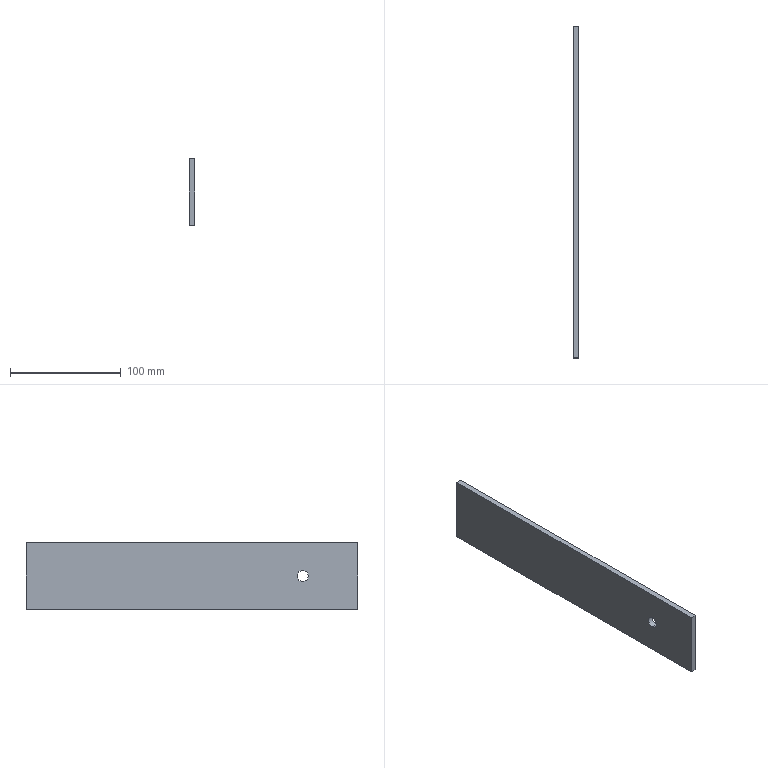Part | SolidWorks | features Extrusion 1, ICE 1 | 1 solid | 8 faces | box 5 x 300 x 60 mm | volume 89607 mm3 | plane 6 | cylinder 2 | commonest cylinder face diameters 10 x2
STEP:
#1=CARTESIAN_POINT('',(-2.5,-100.,35.));
#2=VERTEX_POINT('',#1);
#3=CARTESIAN_POINT('',(-2.5,-100.,25.));
#4=VERTEX_POINT('',#3);
#5=CARTESIAN_POINT('',(-2.5,-100.,30.));
#6=DIRECTION('',(1.,0.,0.));
#7=DIRECTION('',(0.,0.,-1.));
#8=AXIS2_PLACEMENT_3D('',#5,#6,#7);
#9=CIRCLE('',#8,5.);
#10=EDGE_CURVE('',#2,#4,#9,.T.);
#11=ORIENTED_EDGE('',*,*,#10,.F.);
#12=CARTESIAN_POINT('',(2.5,-100.,35.));
#13=VERTEX_POINT('',#12);
#14=CARTESIAN_POINT('',(-17.5,-100.,35.));
#15=DIRECTION('',(1.,0.,0.));
#16=VECTOR('',#15,1000.);
#17=LINE('',#14,#16);
#18=EDGE_CURVE('',#2,#13,#17,.T.);
#19=ORIENTED_EDGE('',*,*,#18,.T.);
#20=CARTESIAN_POINT('',(2.5,-100.,25.));
#21=VERTEX_POINT('',#20);
#22=CARTESIAN_POINT('',(2.5,-100.,30.));
#23=DIRECTION('',(1.,0.,0.));
#24=DIRECTION('',(0.,0.,-1.));
#25=AXIS2_PLACEMENT_3D('',#22,#23,#24);
#26=CIRCLE('',#25,5.);
#27=EDGE_CURVE('',#13,#21,#26,.T.);
#28=ORIENTED_EDGE('',*,*,#27,.T.);
#29=CARTESIAN_POINT('',(-17.5,-100.,25.));
#30=DIRECTION('',(1.,0.,0.));
#31=VECTOR('',#30,1000.);
#32=LINE('',#29,#31);
#33=EDGE_CURVE('',#4,#21,#32,.T.);
#34=ORIENTED_EDGE('',*,*,#33,.F.);
#35=EDGE_LOOP('',(#11,#19,#28,#34));
#36=FACE_OUTER_BOUND('',#35,.T.);
#37=CARTESIAN_POINT('',(-17.5,-100.,30.));
#38=DIRECTION('',(1.,0.,0.));
#39=DIRECTION('',(0.,0.,-1.));
#40=AXIS2_PLACEMENT_3D('',#37,#38,#39);
#41=CYLINDRICAL_SURFACE('',#40,5.);
#42=ADVANCED_FACE('',(#36),#41,.F.);
#43=CARTESIAN_POINT('',(2.5,-100.,30.));
#44=DIRECTION('',(1.,0.,0.));
#45=DIRECTION('',(0.,0.,-1.));
#46=AXIS2_PLACEMENT_3D('',#43,#44,#45);
#47=CIRCLE('',#46,5.);
#48=EDGE_CURVE('',#21,#13,#47,.T.);
#49=ORIENTED_EDGE('',*,*,#48,.F.);
#50=ORIENTED_EDGE('',*,*,#27,.F.);
#51=EDGE_LOOP('',(#49,#50));
#52=FACE_BOUND('',#51,.T.);
#53=CARTESIAN_POINT('',(2.5,-150.,0.));
#54=VERTEX_POINT('',#53);
#55=CARTESIAN_POINT('',(2.5,150.,0.));
#56=VERTEX_POINT('',#55);
#57=CARTESIAN_POINT('',(2.5,-150.,0.));
#58=DIRECTION('',(0.,1.,0.));
#59=VECTOR('',#58,1000.);
#60=LINE('',#57,#59);
#61=EDGE_CURVE('',#54,#56,#60,.T.);
#62=ORIENTED_EDGE('',*,*,#61,.T.);
#63=CARTESIAN_POINT('',(2.5,150.,60.));
#64=VERTEX_POINT('',#63);
#65=CARTESIAN_POINT('',(2.5,150.,60.));
#66=DIRECTION('',(0.,0.,-1.));
#67=VECTOR('',#66,1000.);
#68=LINE('',#65,#67);
#69=EDGE_CURVE('',#64,#56,#68,.T.);
#70=ORIENTED_EDGE('',*,*,#69,.F.);
#71=CARTESIAN_POINT('',(2.5,-150.,60.));
#72=VERTEX_POINT('',#71);
#73=CARTESIAN_POINT('',(2.5,-150.,60.));
#74=DIRECTION('',(0.,1.,0.));
#75=VECTOR('',#74,1000.);
#76=LINE('',#73,#75);
#77=EDGE_CURVE('',#72,#64,#76,.T.);
#78=ORIENTED_EDGE('',*,*,#77,.F.);
#79=CARTESIAN_POINT('',(2.5,-150.,60.));
#80=DIRECTION('',(0.,0.,-1.));
#81=VECTOR('',#80,1000.);
#82=LINE('',#79,#81);
#83=EDGE_CURVE('',#72,#54,#82,.T.);
#84=ORIENTED_EDGE('',*,*,#83,.T.);
#85=EDGE_LOOP('',(#62,#70,#78,#84));
#86=FACE_OUTER_BOUND('',#85,.T.);
#87=CARTESIAN_POINT('',(2.5,-150.,60.));
#88=DIRECTION('',(-1.,0.,0.));
#89=DIRECTION('',(0.,0.,1.));
#90=AXIS2_PLACEMENT_3D('',#87,#88,#89);
#91=PLANE('',#90);
#92=ADVANCED_FACE('',(#52,#86),#91,.F.);
#93=CARTESIAN_POINT('',(-2.5,150.,0.));
#94=VERTEX_POINT('',#93);
#95=CARTESIAN_POINT('',(-2.5,150.,0.));
#96=DIRECTION('',(-1.,0.,0.));
#97=VECTOR('',#96,1000.);
#98=LINE('',#95,#97);
#99=EDGE_CURVE('',#56,#94,#98,.T.);
#100=ORIENTED_EDGE('',*,*,#99,.T.);
#101=CARTESIAN_POINT('',(-2.5,150.,60.));
#102=VERTEX_POINT('',#101);
#103=CARTESIAN_POINT('',(-2.5,150.,60.));
#104=DIRECTION('',(0.,0.,-1.));
#105=VECTOR('',#104,1000.);
#106=LINE('',#103,#105);
#107=EDGE_CURVE('',#102,#94,#106,.T.);
#108=ORIENTED_EDGE('',*,*,#107,.F.);
#109=CARTESIAN_POINT('',(-2.5,150.,60.));
#110=DIRECTION('',(-1.,0.,0.));
#111=VECTOR('',#110,1000.);
#112=LINE('',#109,#111);
#113=EDGE_CURVE('',#64,#102,#112,.T.);
#114=ORIENTED_EDGE('',*,*,#113,.F.);
#115=ORIENTED_EDGE('',*,*,#69,.T.);
#116=EDGE_LOOP('',(#100,#108,#114,#115));
#117=FACE_OUTER_BOUND('',#116,.T.);
#118=CARTESIAN_POINT('',(-2.5,150.,60.));
#119=DIRECTION('',(0.,-1.,0.));
#120=DIRECTION('',(0.,0.,-1.));
#121=AXIS2_PLACEMENT_3D('',#118,#119,#120);
#122=PLANE('',#121);
#123=ADVANCED_FACE('',(#117),#122,.F.);
#124=CARTESIAN_POINT('',(-2.5,-100.,30.));
#125=DIRECTION('',(1.,0.,0.));
#126=DIRECTION('',(0.,0.,-1.));
#127=AXIS2_PLACEMENT_3D('',#124,#125,#126);
#128=CIRCLE('',#127,5.);
#129=EDGE_CURVE('',#4,#2,#128,.T.);
#130=ORIENTED_EDGE('',*,*,#129,.T.);
#131=ORIENTED_EDGE('',*,*,#10,.T.);
#132=EDGE_LOOP('',(#130,#131));
#133=FACE_BOUND('',#132,.T.);
#134=CARTESIAN_POINT('',(-2.5,-150.,0.));
#135=VERTEX_POINT('',#134);
#136=CARTESIAN_POINT('',(-2.5,-150.,0.));
#137=DIRECTION('',(0.,-1.,0.));
#138=VECTOR('',#137,1000.);
#139=LINE('',#136,#138);
#140=EDGE_CURVE('',#94,#135,#139,.T.);
#141=ORIENTED_EDGE('',*,*,#140,.T.);
#142=CARTESIAN_POINT('',(-2.5,-150.,60.));
#143=VERTEX_POINT('',#142);
#144=CARTESIAN_POINT('',(-2.5,-150.,60.));
#145=DIRECTION('',(0.,0.,-1.));
#146=VECTOR('',#145,1000.);
#147=LINE('',#144,#146);
#148=EDGE_CURVE('',#143,#135,#147,.T.);
#149=ORIENTED_EDGE('',*,*,#148,.F.);
#150=CARTESIAN_POINT('',(-2.5,-150.,60.));
#151=DIRECTION('',(0.,-1.,0.));
#152=VECTOR('',#151,1000.);
#153=LINE('',#150,#152);
#154=EDGE_CURVE('',#102,#143,#153,.T.);
#155=ORIENTED_EDGE('',*,*,#154,.F.);
#156=ORIENTED_EDGE('',*,*,#107,.T.);
#157=EDGE_LOOP('',(#141,#149,#155,#156));
#158=FACE_OUTER_BOUND('',#157,.T.);
#159=CARTESIAN_POINT('',(-2.5,-150.,60.));
#160=DIRECTION('',(1.,0.,0.));
#161=DIRECTION('',(0.,0.,-1.));
#162=AXIS2_PLACEMENT_3D('',#159,#160,#161);
#163=PLANE('',#162);
#164=ADVANCED_FACE('',(#133,#158),#163,.F.);
#165=CARTESIAN_POINT('',(-2.5,-150.,0.));
#166=DIRECTION('',(1.,0.,0.));
#167=VECTOR('',#166,1000.);
#168=LINE('',#165,#167);
#169=EDGE_CURVE('',#135,#54,#168,.T.);
#170=ORIENTED_EDGE('',*,*,#169,.T.);
#171=ORIENTED_EDGE('',*,*,#83,.F.);
#172=CARTESIAN_POINT('',(-2.5,-150.,60.));
#173=DIRECTION('',(1.,0.,0.));
#174=VECTOR('',#173,1000.);
#175=LINE('',#172,#174);
#176=EDGE_CURVE('',#143,#72,#175,.T.);
#177=ORIENTED_EDGE('',*,*,#176,.F.);
#178=ORIENTED_EDGE('',*,*,#148,.T.);
#179=EDGE_LOOP('',(#170,#171,#177,#178));
#180=FACE_OUTER_BOUND('',#179,.T.);
#181=CARTESIAN_POINT('',(-2.5,-150.,60.));
#182=DIRECTION('',(0.,1.,0.));
#183=DIRECTION('',(0.,0.,1.));
#184=AXIS2_PLACEMENT_3D('',#181,#182,#183);
#185=PLANE('',#184);
#186=ADVANCED_FACE('',(#180),#185,.F.);
#187=ORIENTED_EDGE('',*,*,#77,.T.);
#188=ORIENTED_EDGE('',*,*,#113,.T.);
#189=ORIENTED_EDGE('',*,*,#154,.T.);
#190=ORIENTED_EDGE('',*,*,#176,.T.);
#191=EDGE_LOOP('',(#187,#188,#189,#190));
#192=FACE_OUTER_BOUND('',#191,.T.);
#193=CARTESIAN_POINT('',(0.,0.,60.));
#194=DIRECTION('',(0.,0.,-1.));
#195=DIRECTION('',(-1.,0.,0.));
#196=AXIS2_PLACEMENT_3D('',#193,#194,#195);
#197=PLANE('',#196);
#198=ADVANCED_FACE('',(#192),#197,.F.);
#199=ORIENTED_EDGE('',*,*,#61,.F.);
#200=ORIENTED_EDGE('',*,*,#169,.F.);
#201=ORIENTED_EDGE('',*,*,#140,.F.);
#202=ORIENTED_EDGE('',*,*,#99,.F.);
#203=EDGE_LOOP('',(#199,#200,#201,#202));
#204=FACE_OUTER_BOUND('',#203,.T.);
#205=CARTESIAN_POINT('',(0.,0.,0.));
#206=DIRECTION('',(0.,0.,-1.));
#207=DIRECTION('',(-1.,0.,0.));
#208=AXIS2_PLACEMENT_3D('',#205,#206,#207);
#209=PLANE('',#208);
#210=ADVANCED_FACE('',(#204),#209,.T.);
#211=ORIENTED_EDGE('',*,*,#18,.F.);
#212=ORIENTED_EDGE('',*,*,#129,.F.);
#213=ORIENTED_EDGE('',*,*,#33,.T.);
#214=ORIENTED_EDGE('',*,*,#48,.T.);
#215=EDGE_LOOP('',(#211,#212,#213,#214));
#216=FACE_OUTER_BOUND('',#215,.T.);
#217=CARTESIAN_POINT('',(-17.5,-100.,30.));
#218=DIRECTION('',(1.,0.,0.));
#219=DIRECTION('',(0.,0.,-1.));
#220=AXIS2_PLACEMENT_3D('',#217,#218,#219);
#221=CYLINDRICAL_SURFACE('',#220,5.);
#222=ADVANCED_FACE('',(#216),#221,.F.);
#223=CLOSED_SHELL('',(#42,#92,#123,#164,#186,#198,#210,#222));
#224=MANIFOLD_SOLID_BREP('',#223);
#225=CARTESIAN_POINT('',(0.,0.,0.));
#226=DIRECTION('',(0.,0.,1.));
#227=DIRECTION('',(1.,0.,0.));
#228=AXIS2_PLACEMENT_3D('',#225,#226,#227);
#229=(LENGTH_UNIT()NAMED_UNIT(*)SI_UNIT(.MILLI.,.METRE.));
#230=UNCERTAINTY_MEASURE_WITH_UNIT(LENGTH_MEASURE(0.00001),#229,'','');
#231=(NAMED_UNIT(*)PLANE_ANGLE_UNIT()SI_UNIT($,.RADIAN.));
#232=(NAMED_UNIT(*)SI_UNIT($,.STERADIAN.)SOLID_ANGLE_UNIT());
#233=(GEOMETRIC_REPRESENTATION_CONTEXT(3)GLOBAL_UNCERTAINTY_ASSIGNED_CONTEXT((#230))GLOBAL_UNIT_ASSIGNED_CONTEXT((#229,#231,#232))REPRESENTATION_CONTEXT('',''));
#234=ADVANCED_BREP_SHAPE_REPRESENTATION('',(#224,#228),#233);